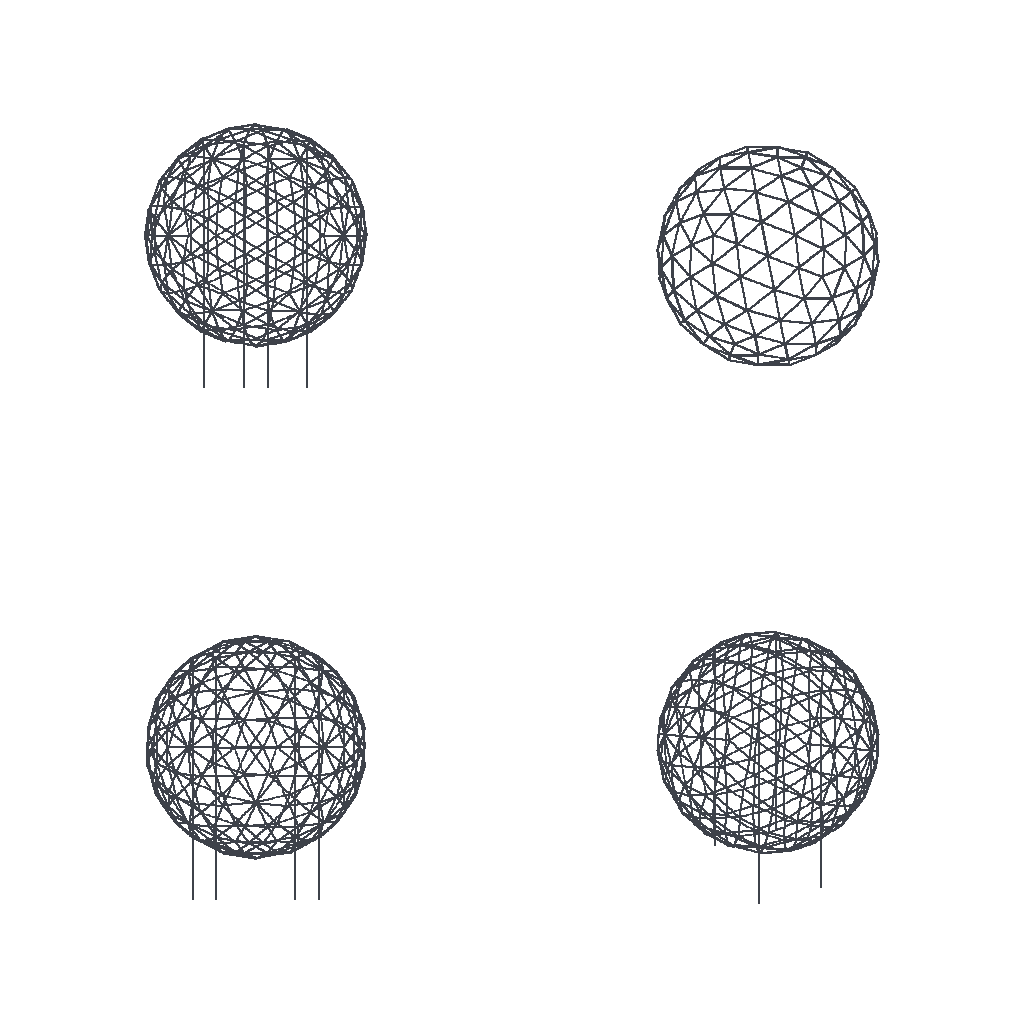Simulation study | abaqus
Set-up summary:
category,name,step,type,value,unit,region
solver,abaqus
solver,version,,,Abaqus/Standard 2020
units,not stated in the deck,,not stated
analysis,deck,,buckling,buckling
load_step,Step-1,Step-1,buckling,nlgeom=False
contact,interactions,,,general=0 pairs=0 ties=0
load_step,requested,,,1
mesh,nodes,,,12925
mesh,elements,,,13240
element_type,B31,,beam,13240
load,load commands in deck,,count,1
bc,support commands in deck,,count,2
material,ALUMINIUM,,in results
material,BPC,,in results
material,BPC_1,,in results
material,Q235,,in results
material,SI_MM111111_Q345,,in results
check,setup vs results,,match,"per instance, exact: element labels, types and connectivity; labels of the nodes the elements use; coordinates of those nodes at SINGLE_PRECISION in 1 of 1 instance(s)"
Abaqus input file, long lists of numbers shortened, first 1045 of 4413 lines:
*Heading
** Job name: Job-1 Model name: Job-4
** Generated by: Abaqus/CAE 2020
*Preprint, echo=NO, model=NO, history=NO, contact=NO
**
** PARTS
**
*Part, name=Part-1
*Node
      1,  -2639.88,     -2027.63,  -1081.56
      2,  -2661.068,  -2001.274,  -1059.834
** (12923 more lines like these left out)
*Element, type=B31
  1, 6026, 6027
  2, 6027, 6028
** (13238 more lines like these left out)
*Nset, nset=_PICKEDSET2_#1, internal
 5761, 5762, 5763, 5764, 5765, 5766, 5767, 5768, 5769, 5770, 5771, 5772, 5773, 5774, 5775, 5776
 5777, 5778, 5779, 5780, 5781, 5782, 5783, 5784, 5785, 5786, 5787, 5788, 5789, 5790, 5791, 5792
** (10 more lines like these left out)
*Elset, elset=_PICKEDSET2_#1, internal, generate
   1,  190,    1
*Nset, nset=_PICKEDSET2_#2, internal
 9114, 9115, 9116, 9117, 9118, 9119, 9120, 9121, 9122, 9123, 9124, 9125, 9126, 9127, 9128, 9129
 9130, 9131, 9132, 9133, 9134, 9135, 9136, 9137, 9138, 9139, 9140, 9141, 9142, 9143, 9144, 9145
** (10 more lines like these left out)
*Elset, elset=_PICKEDSET2_#2, internal, generate
 191,  380,    1
*Nset, nset=_PICKEDSET2_#3, internal
 6823, 6824, 6825, 6826, 6827, 6828, 6829, 6830, 6831, 6832, 6833, 6834, 6835, 6836, 6837, 6838
 6839, 6840, 6841, 6842, 6843, 6844, 6845, 6846, 6847, 6848, 6849, 6850, 6851, 6852, 6853, 6854
** (10 more lines like these left out)
*Elset, elset=_PICKEDSET2_#3, internal, generate
 381,  570,    1
*Nset, nset=_PICKEDSET2_#4, internal
 3484, 3485, 3486, 3487, 3488, 3489, 3490, 3491, 3492, 3493, 3494, 3495, 3496, 3497, 3498, 3499
 3500, 3501, 3502, 3503, 3504, 3505, 3506, 3507, 3508, 3509, 3510, 3511, 3512, 3513, 3514, 3515
** (10 more lines like these left out)
*Elset, elset=_PICKEDSET2_#4, internal, generate
 571,  760,    1
*Nset, nset=SET-1
 6101, 6102, 6103, 6104, 6105, 6106, 6107, 6108, 6109, 6110, 6111, 6112, 6113, 6114, 6115, 6116
 6117, 7798, 7799, 7842, 7843, 7844, 7845, 7846, 7847, 7848, 7849
*Elset, elset=SET-1, generate
 761,  786,    1
*Nset, nset=SET-2
 6166, 6167, 6168, 6169, 6170, 6171, 6172, 6173, 6174, 6175, 6176, 6177, 6178, 6179, 6180, 6181
 6182, 6183, 7842, 7850, 7851, 7852, 7853, 7854, 7855, 7856, 7857
*Elset, elset=SET-2, generate
 787,  812,    1
*Nset, nset=SET-3
 7842, 7858, 7859, 7860, 7861, 7862, 7863, 7864, 7865, 7866, 7867, 7868, 7869, 7870, 7871, 7872
 7873, 7874, 7875, 7876, 7877, 7878, 7879, 7880, 7928, 7929, 7930
*Elset, elset=SET-3, generate
 813,  838,    1
*Nset, nset=SET-4
 7842, 7881, 7882, 7883, 7884, 7885, 7886, 7887, 7888, 7889, 7890, 7891, 7892, 7893, 7894, 7895
 7896, 9659, 9660, 9661, 9662, 9663, 9664, 9665, 9666, 9667, 9668
*Elset, elset=SET-4, generate
 839,  864,    1
*Nset, nset=SET-5
 7661, 7662, 7663, 7800, 7801, 7802, 7803, 7804, 7805, 7806, 7807, 7808, 7809, 7810, 7811, 7812
 7813, 7814, 7815, 7816, 7817, 7818, 7842, 7897, 7898, 7899, 7900
*Elset, elset=SET-5, generate
 865,  890,    1
*Nset, nset=SET-6
 7819, 7820, 7821, 7822, 7823, 7824, 7842, 7901, 7902, 7903, 7904, 7905, 7906, 7907, 7908, 7909
 7910, 9625, 9626, 9627, 9628, 9629, 9630
*Elset, elset=SET-6, generate
 891,  912,    1
*Nset, nset=SET-7
 7663, 7664, 7665, 7666, 7667, 7825, 7826, 7827, 7828, 7829, 7830, 7831, 7832, 7833, 7834, 7835
 9625, 9631, 9632, 9633, 9634, 9635, 9636
*Elset, elset=SET-7, generate
 913,  934,    1
*Nset, nset=SET-8
 9447, 9448, 9449, 9450, 9451, 9452, 9453, 9454, 9455, 9456, 9457, 9458, 9459, 9460, 9461, 9625
 9637, 9638, 9639, 9640, 9641, 9642, 9643
*Elset, elset=SET-8, generate
 935,  956,    1
*Nset, nset=SET-9
  9532,  9533,  9625,  9644,  9645,  9646,  9647,  9648,  9649,  9650,  9651,  9652,  9653,  9654,  9669,  9670
  9671,  9672,  9673,  9674, 11070, 11071, 11072
*Elset, elset=SET-9, generate
 957,  978,    1
*Nset, nset=SET-10
 9625, 9655, 9656, 9657, 9658, 9668, 9675, 9676, 9677, 9678, 9679, 9680, 9681, 9682, 9683, 9684
 9685, 9686, 9687, 9688, 9689, 9690, 9691
*Elset, elset=SET-10, generate
  979,  1000,     1
*Nset, nset=SET-11
  9668,  9692,  9693,  9694,  9695,  9696,  9697,  9698,  9699,  9700,  9701,  9702,  9703,  9704,  9705,  9706
  9707,  9708,  9709,  9710,  9711,  9712, 11070, 11073, 11074, 11300, 11301
*Elset, elset=SET-11, generate
 1001,  1026,     1
*Nset, nset=SET-12
 10081, 10082, 10083, 10084, 10085, 10086, 10087, 10088, 10089, 10371, 10372, 10373, 10374, 10375, 10376, 10377
 10378, 10379, 10380, 11566, 11567, 11568, 11569, 11570, 11571, 11572, 11573, 11574
*Elset, elset=SET-12, generate
 1027,  1053,     1
*Nset, nset=SET-13
 10081, 10090, 10091, 10092, 10093, 10094, 10095, 10096, 10097, 10098, 10099, 10100, 10381, 10382, 10383, 10384
 10385, 10386, 10387, 10388, 10389, 10390, 10391, 10392, 10393, 10394, 10395
*Elset, elset=SET-13, generate
 1054,  1079,     1
*Nset, nset=SET-14
  8460,  8461,  8462,  8463,  8464,  8465,  8466,  8467,  8468,  8469,  8470, 10081, 10101, 10102, 10103, 10104
 10105, 10106, 10107, 10108, 10109, 10110, 10111, 10112, 10113, 10114, 10115, 10116
*Elset, elset=SET-14, generate
 1080,  1106,     1
*Nset, nset=SET-15
  8168,  8169,  8170,  8171,  8172,  8173,  8174,  8175,  8547, 10081, 10117, 10118, 10119, 10120, 10121, 10122
 10126, 10127, 10128, 10129, 10130, 10131, 10132, 10133, 10134, 10135, 10136, 10137
*Elset, elset=SET-15, generate
 1107,  1133,     1
*Nset, nset=SET-16
 11574, 11575, 11576, 11577, 11578, 11599, 11600, 11601, 11602, 11603, 11604, 11605, 11606, 11607, 11608, 11609
 11610, 11611, 11612, 11613, 11614, 11615, 11616, 11617, 11618, 11619, 11620, 11621, 11622
*Elset, elset=SET-16, generate
 1134,  1161,     1
*Nset, nset=SET-17
 10081, 10123, 10124, 10138, 10139, 10140, 10141, 10142, 10143, 10144, 10145, 10146, 10147, 10148, 10149, 11439
 11440, 11441, 11442, 11443, 11444, 11445, 11446, 11447, 11448, 11449, 11450, 11599
*Elset, elset=SET-17, generate
 1162,  1188,     1
*Nset, nset=SET-18
 10081, 10125, 10150, 10151, 10152, 10153, 10154, 10155, 10156, 10157, 10158, 10159, 10160, 10161, 10162, 10163
 10164, 10165, 10166, 10167, 10168, 10169, 10170, 10171, 10172, 10173, 10174
*Elset, elset=SET-18, generate
 1189,  1214,     1
*Nset, nset=SET-19
  8168,  8176,  8177,  8178,  8179,  8180,  8181,  8182,  9958,  9959,  9960,  9961,  9962,  9963,  9964,  9965
  9966,  9967,  9968,  9969,  9970, 10150, 10175, 10176, 10177, 10178, 10179
*Elset, elset=SET-19, generate
 1215,  1240,     1
*Nset, nset=SET-20
 8251, 8252, 8253, 8254, 8255, 8256, 8257, 8258, 8259, 9984, 9985, 9986, 9987, 9988, 9989, 9990
 9991, 9992, 9993, 9994, 9995, 9996, 9997
*Elset, elset=SET-20, generate
 1241,  1262,     1
*Nset, nset=SET-21
  9984,  9998,  9999, 10000, 10001, 10002, 10003, 10004, 10005, 10006, 10007, 10008, 10009, 10010, 10011, 10012
 10013, 10014, 10150, 10180, 10181, 10182, 10183
*Elset, elset=SET-21, generate
 1263,  1284,     1
*Nset, nset=SET-22
 10150, 10184, 10185, 10186, 10187, 10188, 10205, 10206, 10207, 10208, 10209, 10210, 10211, 10212, 10213, 10214
 10215, 10216, 10217, 11469, 11470, 11471, 11472, 11473, 11474, 11475, 11476
*Elset, elset=SET-22, generate
 1285,  1310,     1
*Nset, nset=SET-23
 11451, 11452, 11453, 11454, 11455, 11456, 11457, 11469, 11477, 11478, 11479, 11480, 11481, 11482, 11483, 11484
 11485, 11486, 11487, 11488, 11489, 11490, 11491, 11492, 11493, 11494, 11599
*Elset, elset=SET-23, generate
 1311,  1336,     1
*Nset, nset=SET-24
  9984, 10015, 10016, 10017, 10018, 10019, 10020, 10021, 10022, 10023, 10024, 10046, 10047, 10048, 10049, 10050
 10051, 10052, 10234, 10235, 10236, 10237, 10238
*Elset, elset=SET-24, generate
 1337,  1358,     1
*Nset, nset=SET-25
  8334,  8335,  8336,  8337,  8338,  8339,  8340,  8341,  8342, 10053, 10054, 10055, 10056, 10057, 10058, 10059
 10060, 10061, 10062, 10063, 10064, 10065, 10066, 10067, 10234, 10239, 10240
*Elset, elset=SET-25, generate
 1359,  1384,     1
*Nset, nset=SET-26
 10218, 10219, 10220, 10221, 10222, 10234, 10241, 10242, 10243, 10244, 10245, 10246, 10247, 10248, 10249, 10250
 10251, 10252, 10253, 11469, 11495, 11496, 11497, 11498, 11499, 11500, 11501
*Elset, elset=SET-26, generate
 1385,  1410,     1
*Nset, nset=SET-27
 11469, 11502, 11503, 11504, 11505, 11506, 11507, 11508, 11509, 11510, 11511, 11528, 11529, 11530, 11531, 11532
 11533, 11534, 11535, 11536, 11537, 11538, 11539, 11540, 11541, 11542, 11742
*Elset, elset=SET-27, generate
 1411,  1436,     1
*Nset, nset=SET-28
 11599, 11623, 11624, 11625, 11626, 11627, 11628, 11629, 11661, 11662, 11663, 11664, 11665, 11666, 11667, 11668
 11669, 11670, 11671, 11672, 11673, 11674, 11675, 11676, 11677, 11678, 11679, 11680
*Elset, elset=SET-28, generate
 1437,  1463,     1
*Nset, nset=SET-29
 11661, 11681, 11682, 11683, 11684, 11685, 11686, 11687, 11688, 11689, 11690, 11691, 11692, 11693, 11694, 11695
 11696, 11697, 11896, 11897, 11898, 11899, 11900, 11901, 11902, 11903, 11970, 11971
*Elset, elset=SET-29, generate
 1464,  1490,     1
*Nset, nset=SET-30
 11661, 11698, 11699, 11700, 11701, 11702, 11703, 11704, 11705, 11706, 11707, 11708, 11742, 11743, 11744, 11745
 11746, 11747, 11748, 11749, 11750, 11751, 11752, 11753, 11754, 11755, 11756, 11757
*Elset, elset=SET-30, generate
 1491,  1517,     1
*Nset, nset=SET-31
 11661, 11709, 11710, 11711, 11712, 11713, 11714, 11715, 11716, 11717, 11718, 11719, 11758, 11759, 11760, 11761
 11762, 11763, 12040, 12041, 12042, 12043, 12044, 12045, 12046, 12047, 12048, 12049
*Elset, elset=SET-31, generate
 1518,  1544,     1
*Nset, nset=SET-32
 10234, 10254, 10255, 10256, 10257, 10258, 10259, 10260, 10261, 10262, 10263, 10264, 10265, 10266, 10267, 10268
 10269, 10293, 10294, 10295, 10296, 10297, 10298, 10299, 10300, 10301, 10302
*Elset, elset=SET-32, generate
 1545,  1570,     1
*Nset, nset=SET-33
 10270, 10271, 10272, 10273, 10293, 10303, 10304, 10305, 10306, 10307, 10308, 10309, 10310, 10311, 10312, 11543
 11544, 11545, 11546, 11547, 11548, 11549, 11550, 11551, 11552, 11553, 11554, 11742
*Elset, elset=SET-33, generate
 1571,  1597,     1
*Nset, nset=SET-34
 11742, 11764, 11765, 11766, 11767, 11768, 11769, 11770, 11771, 11772, 11773, 11774, 11775, 11776, 11777, 11778
 11802, 11803, 11804, 11805, 11806, 11807, 11808, 11809, 11810, 11811, 11812, 11813, 11814
*Elset, elset=SET-34, generate
 1598,  1625,     1
*Nset, nset=SET-35
 11742, 11779, 11780, 11781, 11782, 11783, 11784, 11785, 11786, 11787, 11788, 11789, 11790, 11791, 11792, 11793
 11794, 11795, 11796, 11797, 11798, 11799, 11800, 12040, 12050, 12051, 12052, 12053, 12054
*Elset, elset=SET-35, generate
 1626,  1653,     1
*Nset, nset=SET-36
 10234, 10274, 10275, 10276, 10277, 10278, 10279, 10280, 10281, 10282, 10283, 10284, 10285, 10286, 10287, 11555
 11556, 11557, 11558, 11559, 11560, 11561, 11562, 11563, 11564, 11565, 11742
*Elset, elset=SET-36, generate
 1654,  1679,     1
*Nset, nset=SET-37
  8343,  8344,  8345,  8346,  8347,  8419,  8420,  8421, 10068, 10069, 10070, 10071, 10072, 10073, 10074, 10075
 10076, 10077, 10078, 10079, 10080, 10234, 10288, 10289, 10290, 10291, 10292
*Elset, elset=SET-37, generate
 1680,  1705,     1
*Nset, nset=SET-38
 11661, 11720, 11721, 11722, 11723, 11724, 11725, 11726, 11727, 11728, 11972, 11973, 11974, 11975, 11976, 11977
 11978, 11979, 11980, 11981, 11982, 11983, 11984, 11985, 11986, 11987, 11988
*Elset, elset=SET-38, generate
 1706,  1731,     1
*Nset, nset=SET-39
 11469, 11512, 11513, 11514, 11515, 11516, 11517, 11518, 11519, 11520, 11521, 11522, 11523, 11661, 11729, 11730
 11731, 11732, 11733, 11734, 11735, 11736, 11737, 11738, 11739, 11740, 11741
*Elset, elset=SET-39, generate
 1732,  1757,     1
*Nset, nset=SET-40
  9984, 10025, 10026, 10027, 10028, 10029, 10030, 10223, 10224, 10225, 10226, 10227, 10228, 10229, 10230, 10231
 10232, 10233, 11469, 11524, 11525, 11526, 11527
*Elset, elset=SET-40, generate
 1758,  1779,     1
*Nset, nset=SET-41
  8260,  8261,  8262,  8334,  8348,  8349,  8350,  8351,  8352,  9984, 10031, 10032, 10033, 10034, 10035, 10036
 10037, 10038, 10039, 10040, 10041, 10042, 10043
*Elset, elset=SET-41, generate
 1780,  1801,     1
*Nset, nset=SET-42
 11599, 11630, 11631, 11632, 11633, 11634, 11635, 11636, 11637, 11638, 11639, 11640, 11641, 11642, 11643, 11644
 11645, 11646, 11647, 11648, 11649, 11650, 11651, 11903, 11904, 11905, 11906, 11907, 11908
*Elset, elset=SET-42, generate
 1802,  1829,     1
*Nset, nset=SET-43
 10150, 10189, 10190, 10191, 10192, 10193, 10194, 10195, 10196, 10197, 10198, 10199, 10200, 10201, 10202, 11458
 11459, 11460, 11461, 11462, 11463, 11464, 11465, 11466, 11467, 11468, 11599
*Elset, elset=SET-43, generate
 1830,  1855,     1
*Nset, nset=SET-44
  8259,  8263,  8264,  8265,  8266,  8267,  8268,  8269,  8270,  9971,  9972,  9973,  9974,  9975,  9976,  9977
  9978,  9979,  9980,  9981,  9982,  9983, 10044, 10045, 10150, 10203, 10204
*Elset, elset=SET-44, generate
 1856,  1881,     1
*Nset, nset=SET-45
 6183, 6184, 6185, 6186, 6187, 6188, 6189, 6190, 6191, 6192, 6193, 6194, 6195, 6196, 6197, 6198
 6199, 6200, 7911, 7912, 7913, 7914, 7915, 7928, 7931, 7932, 7933, 7934
*Elset, elset=SET-45, generate
 1882,  1908,     1
*Nset, nset=SET-46
  9668,  9713,  9714,  9715,  9716,  9717,  9718,  9719,  9720,  9721,  9722,  9723,  9724,  9725,  9726,  9727
  9728,  9729, 11302, 11303, 11304, 11305, 11328, 11329, 11330, 11331, 11332
*Elset, elset=SET-46, generate
 1909,  1934,     1
*Nset, nset=SET-47
 7916, 7917, 7918, 7919, 7920, 7921, 7922, 7923, 7924, 7925, 7926, 7927, 7928, 7935, 7936, 7937
 7938, 9668, 9730, 9731, 9732, 9733, 9734, 9735, 9736, 9737, 9738
*Elset, elset=SET-47, generate
 1935,  1960,     1
*Nset, nset=SET-48
 9668, 9739, 9740, 9741, 9742, 9743, 9744, 9745, 9746, 9747, 9748, 9749, 9750, 9751, 9752, 9753
 9754, 9755, 9756, 9757, 9758, 9759, 9760, 9761, 9762, 9763, 9764
*Elset, elset=SET-48, generate
 1961,  1986,     1
*Nset, nset=SET-49
  9748,  9765,  9766,  9767,  9768,  9769,  9770,  9771,  9772,  9773,  9774,  9775,  9776,  9777,  9778,  9779
  9780,  9781, 11332, 11333, 11334, 11335, 11336, 11337, 11338, 11339, 11340, 11341
*Elset, elset=SET-49, generate
 1987,  2013,     1
*Nset, nset=SET-50
  9748,  9782,  9783,  9784,  9785,  9786,  9787,  9788,  9789,  9790,  9791,  9792,  9793,  9794,  9795,  9796
  9797,  9798, 11342, 11380, 11381, 11382, 11383, 11384, 11385, 11386, 11387, 11388
*Elset, elset=SET-50, generate
 2014,  2040,     1
*Nset, nset=SET-51
 7928, 7939, 7940, 7941, 7942, 7943, 7944, 7945, 7946, 7947, 7948, 7949, 7950, 7951, 7952, 7953
 7954, 9748, 9799, 9800, 9801, 9802, 9803, 9804, 9805, 9806, 9807, 9808
*Elset, elset=SET-51, generate
 2041,  2067,     1
*Nset, nset=SET-52
 6241, 6242, 6243, 6244, 6245, 6246, 6247, 6248, 6249, 6250, 6251, 6252, 6253, 6254, 6255, 6256
 6257, 6258, 6259, 7928, 7955, 7956, 7957, 7958, 7959, 7960, 7961, 7962, 7963
*Elset, elset=SET-52, generate
 2068,  2095,     1
*Nset, nset=SET-53
 7928, 7964, 7965, 7966, 7967, 7968, 7969, 7970, 7971, 7972, 7973, 7974, 7975, 7976, 7977, 7978
 7979, 7980, 7981, 7982, 7983, 7984, 7985, 7986, 7996, 7997, 7998, 7999, 8000
*Elset, elset=SET-53, generate
 2096,  2123,     1
*Nset, nset=SET-54
 6259, 6260, 6261, 6262, 6263, 6264, 6265, 6266, 6267, 6268, 6269, 6270, 6271, 6272, 6273, 6274
 6275, 6276, 6277, 7987, 7996, 8001, 8002, 8003, 8004, 8005, 8006, 8007, 8008
*Elset, elset=SET-54, generate
 2124,  2151,     1
*Nset, nset=SET-55
 7988, 7989, 7990, 7991, 7992, 7993, 7994, 7995, 7996, 8009, 8010, 8011, 8012, 8013, 8014, 8015
 8016, 9748, 9809, 9810, 9811, 9812, 9813, 9814, 9815, 9816, 9817, 9818
*Elset, elset=SET-55, generate
 2152,  2178,     1
*Nset, nset=SET-56
 9748, 9819, 9820, 9821, 9822, 9823, 9824, 9825, 9826, 9827, 9828, 9829, 9830, 9831, 9832, 9833
 9834, 9835, 9836, 9837, 9838, 9839, 9840, 9841, 9842, 9843, 9844
*Elset, elset=SET-56, generate
 2179,  2204,     1
*Nset, nset=SET-57
  9828,  9845,  9846,  9847,  9848,  9849,  9850,  9851,  9852,  9853,  9854,  9855,  9856,  9857,  9858,  9859
  9860,  9861, 11380, 11389, 11390, 11391, 11392, 11393, 11394, 11395, 11396
*Elset, elset=SET-57, generate
 2205,  2230,     1
*Nset, nset=SET-58
 6315, 6316, 6317, 6318, 6319, 6320, 6321, 6322, 6323, 6324, 6325, 6326, 6327, 6328, 6329, 6330
 6331, 6332, 7996, 8017, 8018, 8019, 8020, 8021, 8022, 8023, 8024, 8025
*Elset, elset=SET-58, generate
 2231,  2257,     1
*Nset, nset=SET-59
 7996, 8026, 8027, 8028, 8029, 8030, 8031, 8032, 8033, 8034, 8035, 8036, 8037, 8038, 8039, 8040
 8041, 8042, 8043, 8044, 8045, 8046, 8047, 8076, 8077, 8078, 8079
*Elset, elset=SET-59, generate
 2258,  2283,     1
*Nset, nset=SET-60
 7996, 8048, 8049, 8050, 8051, 8052, 8053, 8054, 8055, 8056, 8057, 8058, 8059, 8060, 8061, 8062
 8063, 9828, 9862, 9863, 9864, 9865, 9866, 9867, 9868, 9869, 9870
*Elset, elset=SET-60, generate
 2284,  2309,     1
*Nset, nset=SET-61
 8064, 8065, 8066, 8067, 8068, 8069, 8070, 8071, 8072, 8073, 8076, 8080, 8081, 8082, 8083, 8084
 8085, 9828, 9871, 9872, 9873, 9874, 9875, 9876, 9877, 9878, 9879
*Elset, elset=SET-61, generate
 2310,  2335,     1
*Nset, nset=SET-62
 9828, 9880, 9881, 9882, 9883, 9884, 9885, 9886, 9887, 9888, 9889, 9909, 9910, 9911, 9912, 9913
 9914, 9915, 9916, 9917, 9918, 9919, 9920
*Elset, elset=SET-62, generate
 2336,  2357,     1
*Nset, nset=SET-63
  9828,  9890,  9891,  9892,  9893,  9894,  9895,  9896,  9897,  9898,  9899,  9900,  9901,  9902,  9903,  9904
  9905,  9906,  9907,  9908,  9921,  9922, 11224, 11225, 11226, 11437, 11438
*Elset, elset=SET-63, generate
 2358,  2383,     1
*Nset, nset=SET-64
 6462, 6463, 6464, 6465, 6466, 6467, 6468, 6469, 6470, 6471, 8157, 8158, 8159, 8160, 8161, 8162
 8163, 8164, 8165, 8168, 8183, 8184, 8185, 8186, 8187, 8188, 8189, 8190, 8191
*Elset, elset=SET-64, generate
 2384,  2411,     1
*Nset, nset=SET-65
 8166, 8167, 8168, 8192, 8193, 8194, 8195, 8196, 8197, 8470, 8471, 8472, 8473, 8474, 8475, 8476
 8477, 8478, 8479, 8480, 8481, 8482, 8483, 8484, 8485, 8486, 8487, 8488, 8489
*Elset, elset=SET-65, generate
 2412,  2439,     1
*Nset, nset=SET-66
 8334, 8353, 8354, 8355, 8356, 8357, 8358, 8359, 8360, 8361, 8362, 8363, 8364, 8365, 8366, 8367
 8368, 8369, 8370, 8371, 8372, 8373, 8374, 8375, 8376, 8419, 8422
*Elset, elset=SET-66, generate
 2440,  2465,     1
*Nset, nset=SET-67
 6602, 6603, 6604, 6605, 6606, 6607, 6608, 8271, 8272, 8273, 8274, 8275, 8276, 8277, 8278, 8279
 8280, 8281, 8282, 8283, 8334, 8377, 8378, 8379, 8380, 8381, 8382
*Elset, elset=SET-67, generate
 2466,  2491,     1
*Nset, nset=SET-68
 6602, 6609, 6610, 6611, 6612, 6613, 6614, 8259, 8284, 8285, 8286, 8287, 8288, 8289, 8290, 8291
 8292, 8293, 8294, 8295, 8296, 8297, 8298, 8299, 8300, 8301, 8302
*Elset, elset=SET-68, generate
 2492,  2517,     1
*Nset, nset=SET-69
 8168, 8198, 8199, 8200, 8201, 8202, 8203, 8204, 8205, 8206, 8207, 8208, 8209, 8210, 8211, 8212
 8213, 8214, 8215, 8216, 8217, 8218, 8219, 8259, 8303, 8304, 8305
*Elset, elset=SET-69, generate
 2518,  2543,     1
*Nset, nset=SET-70
 8259, 8306, 8307, 8308, 8309, 8310, 8311, 8312, 8313, 8314, 8315, 8316, 8317, 8318, 8319, 8320
 8321, 8322, 8323, 8324, 8325, 8326, 8327, 8334, 8383, 8384, 8385
*Elset, elset=SET-70, generate
 2544,  2569,     1
*Nset, nset=SET-71
 6676, 6677, 6678, 6679, 6680, 6681, 6682, 6683, 8334, 8386, 8387, 8388, 8389, 8390, 8391, 8392
 8393, 8394, 8395, 8396, 8397, 8398, 8399, 8400, 8401, 8402, 8403
*Elset, elset=SET-71, generate
 2570,  2595,     1
*Nset, nset=SET-72
 6527, 6528, 6529, 6530, 6531, 6532, 6533, 6534, 8220, 8221, 8222, 8223, 8224, 8225, 8226, 8227
 8228, 8229, 8230, 8231, 8259, 8328, 8329, 8330, 8331, 8332, 8333
*Elset, elset=SET-72, generate
 2596,  2621,     1
*Nset, nset=SET-73
 6527, 6535, 6536, 6537, 6538, 6539, 6540, 6541, 8168, 8232, 8233, 8234, 8235, 8236, 8237, 8238
 8239, 8240, 8241, 8242, 8243, 8244, 8245, 8246, 8247, 8248, 8249, 8250
*Elset, elset=SET-73, generate
 2622,  2648,     1
*Nset, nset=SET-74
 308, 309, 310, 311, 312, 313, 314, 315, 316, 317, 318, 319, 320, 321, 623, 624
 625, 626, 627, 628, 629, 630, 631, 632, 633, 634, 635
*Elset, elset=SET-74, generate
 2649,  2674,     1
*Nset, nset=SET-75
 308, 322, 323, 324, 325, 326, 327, 328, 329, 330, 331, 332, 333, 334, 335, 336
 337, 338, 339, 340, 341, 342, 343, 344, 345, 393, 394
*Elset, elset=SET-75, generate
 2675,  2700,     1
*Nset, nset=SET-76
 223, 224, 225, 226, 227, 228, 229, 230, 231, 232, 308, 346, 347, 348, 349, 350
 553, 554, 555, 556, 557, 558, 559
*Elset, elset=SET-76, generate
 2701,  2722,     1
*Nset, nset=SET-77
 233, 234, 235, 236, 237, 238, 239, 240, 241, 242, 243, 244, 245, 246, 247, 248
 249, 250, 251, 252, 253, 254, 255, 308, 351, 352, 353
*Elset, elset=SET-77, generate
 2723,  2748,     1
*Nset, nset=SET-78
  32,  33,  34,  35,  36,  37,  38,  39,  40,  41,  42,  43,  44,  45, 256, 257
 258, 259, 260, 261, 308, 354, 355, 356, 357, 358, 359
*Elset, elset=SET-78, generate
 2749,  2774,     1
*Nset, nset=SET-79
  94,  95,  96,  97,  98,  99, 100, 101, 102, 103, 104, 105, 308, 360, 361, 362
 363, 364, 365, 366, 367, 368, 369, 370, 371, 372, 373
*Elset, elset=SET-79, generate
 2775,  2800,     1
*Nset, nset=SET-80
 5696, 5697, 5698, 5699, 5700, 5701, 5702, 7568, 7569, 7570, 7571, 7572, 7573, 7574, 7575, 7576
 7577, 7578, 7579, 7580, 7581, 7582, 7583, 7584, 7585, 7586, 7587, 7588, 7743
*Elset, elset=SET-80, generate
 2801,  2828,     1
*Nset, nset=SET-81
 7461, 7462, 7463, 7464, 7465, 7466, 7589, 7590, 7591, 7592, 7593, 7594, 7595, 7596, 7597, 7598
 7599, 7600, 7601, 7602, 7603, 7604, 7605, 7606, 7607, 7608, 7609, 7610, 7743
*Elset, elset=SET-81, generate
 2829,  2856,     1
*Nset, nset=SET-82
 5702, 5703, 5704, 5705, 5706, 5707, 7461, 7467, 7468, 7469, 7470, 7471, 7472, 7473, 7474, 7475
 7476, 7477, 7478, 7479, 7611, 7612, 7613, 7614, 7615, 7616, 7617, 7618, 7619
*Elset, elset=SET-82, generate
 2857,  2884,     1
*Nset, nset=SET-83
 4379, 4380, 4381, 4382, 4383, 4384, 4385, 4386, 4387, 4388, 4389, 4390, 4391, 4392, 4393, 4394
 4395, 4396, 4397, 4398, 4729, 4730, 4731, 4732, 4733, 4734, 4735, 4736, 4737
*Elset, elset=SET-83, generate
 2885,  2912,     1
*Nset, nset=SET-84
 4729, 4738, 4739, 4740, 4741, 4742, 4743, 4744, 4745, 4746, 4747, 4748, 4749, 4750, 4751, 4752
 4753, 4754, 4755, 6390, 6391, 6392, 6393, 6394, 6395, 6396, 6397, 6398, 6399
*Elset, elset=SET-84, generate
 2913,  2940,     1
*Nset, nset=SET-85
 4398, 4399, 4400, 4401, 4402, 4403, 4404, 4405, 4406, 4407, 4408, 4409, 4410, 4411, 4412, 4413
 4414, 4415, 6017, 6018, 6390, 6400, 6401, 6402, 6403, 6404, 6405, 6406, 6407
*Elset, elset=SET-85, generate
 2941,  2968,     1
*Nset, nset=SET-86
 11332, 11343, 11344, 11345, 11346, 11347, 11348, 11349, 11350, 11351, 11352, 11353, 11354, 11355, 11356, 11357
 11358, 11359, 11360, 11361, 11362, 11363, 11364, 11365, 11380, 11397, 11398, 11399, 11400
*Elset, elset=SET-86, generate
 2969,  2996,     1
*Nset, nset=SET-87
 11149, 11150, 11151, 11152, 11153, 11154, 11155, 11156, 11157, 11158, 11159, 11160, 11161, 11162, 11332, 11366
 11367, 11368, 11369, 11370, 11371, 11372, 11373, 12826, 12827, 12828, 12829, 12830, 12831
*Elset, elset=SET-87, generate
 2997,  3024,     1
*Nset, nset=SET-88
 11163, 11164, 11165, 11166, 11167, 11168, 11169, 11170, 11171, 11172, 11173, 11174, 11175, 11176, 11380, 11401
 11402, 11403, 11404, 11405, 11406, 11407, 11408, 12826, 12832, 12833, 12834, 12835, 12836
*Elset, elset=SET-88, generate
 3025,  3052,     1
*Nset, nset=SET-89
 10802, 10803, 10804, 10805, 10806, 10807, 10954, 10955, 10956, 10957, 10958, 10959, 10960, 10961, 10962, 10963
 10964, 10965, 10966, 10967, 10968, 10969, 10970, 10971, 10972, 10973, 10974, 10975, 11227
*Elset, elset=SET-89, generate
 3053,  3080,     1
*Nset, nset=SET-90
 10976, 10977, 10978, 10979, 10980, 10981, 10982, 10983, 10984, 10985, 10986, 10987, 10988, 10989, 11227, 12755
 12756, 12757, 12758, 12759, 12760, 12761, 12762, 12763, 12764, 12765, 12766, 12767, 12768
*Elset, elset=SET-90, generate
 3081,  3108,     1
*Nset, nset=SET-91
 10807, 10808, 10809, 10810, 10811, 10812, 10813, 10814, 10815, 12439, 12440, 12441, 12442, 12443, 12755, 12769
 12770, 12771, 12772, 12773, 12774, 12775, 12776, 12777, 12778, 12779, 12780, 12781, 12782
*Elset, elset=SET-91, generate
 3109,  3136,     1
*Nset, nset=SET-92
 11801, 11802, 11815, 11816, 11817, 11818, 11819, 11820, 11821, 11822, 11823, 11824, 11825, 11826, 12040, 12055
 12056, 12057, 12058, 12059, 12060, 12061, 12062, 12063, 12064, 12065, 12066, 12067, 12068
*Elset, elset=SET-92, generate
 3137,  3164,     1
*Nset, nset=SET-93
 11574, 11579, 11580, 11581, 11582, 11652, 11653, 11654, 11655, 11656, 11657, 11658, 11659, 11660, 11903, 11909
 11910, 11911, 11912, 11913, 11914, 11915, 11916, 11917, 11918, 11919, 11920, 11921, 11922
*Elset, elset=SET-93, generate
 3165,  3192,     1
*Nset, nset=SET-94
 10744, 10745, 10746, 10747, 10748, 10749, 10750, 10751, 10752, 12169, 12170, 12171, 12172, 12173, 12494, 12495
 12496, 12497, 12498, 12499, 12500, 12501, 12506, 12507, 12508, 12509, 12510, 12511, 12512
*Elset, elset=SET-94, generate
 3193,  3220,     1
*Nset, nset=SET-95
 10885, 10886, 10887, 10888, 10889, 10890, 10891, 10892, 10893, 10894, 10895, 10896, 10897, 10898, 11026, 12502
 12503, 12504, 12505, 12506, 12513, 12514, 12515, 12516, 12517, 12518, 12519, 12520, 12521
*Elset, elset=SET-95, generate
 3221,  3248,     1
*Nset, nset=SET-96
 10752, 10753, 10754, 10755, 10756, 10757, 10899, 10900, 10901, 10902, 10903, 10904, 10905, 10906, 10907, 10908
 10909, 10910, 10911, 10912, 10913, 10914, 10915, 10916, 10917, 10918, 10919, 10920, 11026
*Elset, elset=SET-96, generate
 3249,  3276,     1
*Nset, nset=SET-97
 7412, 7413, 7414, 7415, 7416, 7417, 7510, 7511, 7512, 7513, 7514, 7515, 7516, 7517, 7518, 7519
 7520, 7521, 7522, 7523, 7524, 7525, 7526, 7527, 7528, 7529, 7530, 7531, 7626
*Elset, elset=SET-97, generate
 3277,  3304,     1
*Nset, nset=SET-98
 5631, 5632, 5633, 5634, 5635, 5636, 5637, 7532, 7533, 7534, 7535, 7536, 7537, 7538, 7539, 7540
 7541, 7542, 7543, 7544, 7545, 7546, 7547, 7548, 7549, 7550, 7551, 7552, 7626
*Elset, elset=SET-98, generate
 3305,  3332,     1
*Nset, nset=SET-99
 5129, 5301, 5302, 5303, 5304, 5305, 5306, 5307, 5308, 5309, 5310, 5311, 5312, 5313, 5314, 5315
 5316, 5317, 5318, 5319, 5320, 5321, 5322, 5417, 5418, 5419, 5420, 5421, 5422
*Elset, elset=SET-99, generate
 3333,  3360,     1
*Nset, nset=SET-100
 5129, 5323, 5324, 5325, 5326, 5327, 5328, 5329, 5330, 5331, 5332, 5333, 5334, 5335, 5336, 5337
 5338, 5339, 5340, 5341, 5342, 5343, 7164, 7165, 7166, 7167, 7168, 7169, 7170
*Elset, elset=SET-100, generate
 3361,  3388,     1
*Nset, nset=SET-101
 5344, 5345, 5346, 5347, 5348, 5349, 5350, 5351, 5352, 5422, 5423, 5424, 5425, 5426, 5427, 5428
 5429, 5430, 5431, 5432, 5433, 5434, 5435, 7164, 7171, 7172, 7173, 7174, 7175
*Elset, elset=SET-101, generate
 3389,  3416,     1
*Nset, nset=SET-102
 6471, 6472, 6473, 6474, 6475, 6476, 6477, 6478, 6479, 6946, 6947, 8470, 8490, 8491, 8492, 8493
 8494, 8495, 8496, 8497, 8498, 8499, 8500, 8501, 8502, 8503, 8504, 8505, 8506
*Elset, elset=SET-102, generate
 3417,  3444,     1
*Nset, nset=SET-103
 4900, 4968, 4969, 4970, 4971, 4972, 4973, 4974, 4975, 4976, 6602, 6615, 6616, 6617, 6618, 6619
 6620, 6621, 6622, 6623, 6624, 6625, 6626, 6627, 6628, 6629, 6630, 6631, 6632
*Elset, elset=SET-103, generate
 3445,  3472,     1
*Nset, nset=SET-104
 4901, 4902, 4903, 4904, 4905, 4906, 4907, 4908, 4909, 4910, 6602, 6633, 6634, 6635, 6636, 6637
 6638, 6639, 6640, 6641, 6642, 6643, 6644, 6645, 6646, 6647, 6648, 6649, 6650
*Elset, elset=SET-104, generate
 3473,  3500,     1
*Nset, nset=SET-105
 4901, 4911, 4912, 4913, 4914, 4915, 4916, 4917, 4918, 4919, 4920, 4921, 4922, 4923, 4924, 4925
 4926, 4927, 4928, 4929, 4930, 4931, 4932, 4933, 4976, 4977, 4978, 4979, 4980
*Elset, elset=SET-105, generate
 3501,  3528,     1
*Nset, nset=SET-106
 1516, 1517, 1518, 1519, 1520, 1521, 1522, 1523, 1524, 1525, 1526, 1527, 1528, 1529, 1530, 1531
 1532, 1533, 1534, 1535, 1536, 1537, 1538, 1539, 1568, 1569, 1570, 1571, 1572
*Elset, elset=SET-106, generate
 3529,  3556,     1
*Nset, nset=SET-107
   45,   46,   47,   48,   49,   50, 1516, 1540, 1541, 1542, 1543, 1544, 1545, 1546, 1547, 1750
 1751, 1752, 1753, 1754, 1755, 1756, 1757, 1758, 1759, 1760, 1761, 1762, 1763
*Elset, elset=SET-107, generate
 3557,  3584,     1
*Nset, nset=SET-108
   45,   51,   52,   53,   54,   55, 1572, 1573, 1574, 1575, 1576, 1577, 1578, 1579, 1580, 1764
 1765, 1766, 1767, 1768, 1769, 1770, 1771, 1772, 1773, 1774, 1775, 1776, 1777
*Elset, elset=SET-108, generate
 3585,  3612,     1
*Nset, nset=SET-109
 1825, 1973, 1974, 1975, 1976, 1977, 1978, 1979, 1980, 1981, 1982, 1983, 1984, 1985, 1986, 1987
 1988, 1989, 1990, 1991, 1992, 1993, 1994, 2125, 2126, 2127, 2128, 2129, 2130
*Elset, elset=SET-109, generate
 3613,  3640,     1
*Nset, nset=SET-110
  394,  395,  396,  397,  398,  399,  400,  401,  402,  403,  404,  405,  406,  407, 1825, 1995
 1996, 1997, 1998, 1999, 2000, 2001, 2002, 2003, 2004, 2005, 2006, 2007, 2008
*Elset, elset=SET-110, generate
 3641,  3668,     1
*Nset, nset=SET-111
  394,  408,  409,  410,  411,  412,  413,  414,  415,  416,  417,  418,  419,  420,  421,  703
  704,  705,  706,  707, 2130, 2131, 2132, 2133, 2134, 2135, 2136, 2137, 2138
*Elset, elset=SET-111, generate
 3669,  3696,     1
*Nset, nset=SET-112
 5359, 5360, 5361, 5362, 5363, 5364, 5365, 5366, 5367, 5465, 5466, 5467, 5468, 5469, 5470, 5471
 5472, 5473, 5474, 5475, 5476, 5477, 5478, 7229, 7230, 7231, 7232, 7233, 7234
*Elset, elset=SET-112, generate
 3697,  3724,     1
*Nset, nset=SET-113
 5246, 5368, 5369, 5370, 5371, 5372, 5373, 5374, 5375, 5376, 5377, 5378, 5379, 5380, 5381, 5382
 5383, 5384, 5385, 5386, 5387, 5388, 7229, 7235, 7236, 7237, 7238, 7239, 7240
*Elset, elset=SET-113, generate
 3725,  3752,     1
*Nset, nset=SET-114
 5246, 5389, 5390, 5391, 5392, 5393, 5394, 5395, 5396, 5397, 5398, 5399, 5400, 5401, 5402, 5403
 5404, 5405, 5406, 5407, 5408, 5409, 5410, 5478, 5479, 5480, 5481, 5482, 5483
*Elset, elset=SET-114, generate
 3753,  3780,     1
*Nset, nset=SET-115
 8419, 8423, 8424, 8425, 8426, 8427, 8428, 8429, 8430, 8548, 8549, 8550, 8551, 8552, 8553, 8554
 8555, 8556, 8557, 8558, 8559, 8560, 8561, 8562, 8563, 8564, 8565, 8566, 8567
*Elset, elset=SET-115, generate
 3781,  3808,     1
*Nset, nset=SET-116
 6751, 6752, 6753, 6754, 6755, 6756, 6757, 6758, 6759, 6760, 8419, 8431, 8432, 8433, 8434, 8435
 8436, 8437, 8438, 8439, 8440, 8441, 8442, 8443, 8444, 8445, 8446, 8447, 8448
*Elset, elset=SET-116, generate
 3809,  3836,     1
*Nset, nset=SET-117
 6751, 6761, 6762, 6763, 6764, 6765, 6766, 6767, 6768, 7079, 7080, 8567, 8568, 8569, 8570, 8571
 8572, 8573, 8574, 8575, 8576, 8577, 8578, 8579, 8580, 8581, 8582, 8583, 8584
*Elset, elset=SET-117, generate
 3837,  3864,     1
*Nset, nset=SET-118
  947,  948,  949,  950,  951,  952,  953,  954,  955,  956,  957,  958,  959,  960,  961, 1252
 1312, 1313, 1314, 1315, 1316, 1317, 1318, 1319, 1320, 1321, 1322, 1323, 1324
*Elset, elset=SET-118, generate
 3865,  3892,     1
*Nset, nset=SET-119
  947,  962,  963,  964,  965,  966, 1253, 1254, 1255, 1256, 1257, 1258, 1259, 1260, 1261, 1262
 1263, 1264, 1265, 1266, 1267, 1268, 1269, 1270, 1271, 1272, 1273, 1274, 1275
*Elset, elset=SET-119, generate
 3893,  3920,     1
*Nset, nset=SET-120
 1253, 1276, 1277, 1278, 1279, 1280, 1281, 1282, 1283, 1284, 1285, 1286, 1287, 1288, 1289, 1290
 1324, 1325, 1326, 1327, 1328, 1329, 1330, 1331, 1332, 1333, 1334, 1335, 1336
*Elset, elset=SET-120, generate
 3921,  3948,     1
*Nset, nset=SET-121
 1076, 1077, 1078, 1079, 1080, 1109, 1110, 1111, 1112, 1113, 1114, 1115, 1116, 1117, 1118, 1119
 1120, 1121, 1122, 1123, 1124, 1125, 1126, 1127, 1128, 1129, 1130, 1131, 1132
*Elset, elset=SET-121, generate
 3949,  3976,     1
*Nset, nset=SET-122
  803,  804,  805,  806,  807,  808, 1109, 1133, 1134, 1135, 1136, 1137, 1138, 1139, 1140, 1141
 1142, 1143, 1144, 1145, 1146, 1147, 1148, 1149, 1150, 1151, 1152, 1153, 1154
*Elset, elset=SET-122, generate
 3977,  4004,     1
*Nset, nset=SET-123
  803,  809,  810,  811,  812,  813,  814,  815,  816,  817,  818,  819,  820,  821,  822, 1080
 1081, 1082, 1083, 1084, 1155, 1156, 1157, 1158, 1159, 1160, 1161, 1162, 1163
*Elset, elset=SET-123, generate
 4005,  4032,     1
*Nset, nset=SET-124
 4291, 4292, 4293, 4294, 4295, 4296, 4297, 4298, 4299, 4300, 4301, 4302, 4303, 4304, 4305, 4306
 4307, 4308, 5884, 5885, 6117, 6118, 6119, 6120, 6121, 6122, 6123, 6124, 6125
*Elset, elset=SET-124, generate
 4033,  4060,     1
*Nset, nset=SET-125
 4467, 4468, 4469, 4470, 4471, 4472, 4473, 4474, 4475, 4478, 4479, 4480, 4481, 4482, 4483, 4484
 4485, 4486, 4487, 6117, 6126, 6127, 6128, 6129, 6130, 6131, 6132, 6133, 6134
*Elset, elset=SET-125, generate
 4061,  4088,     1
*Nset, nset=SET-126
 4308, 4309, 4310, 4311, 4312, 4313, 4314, 4315, 4316, 4317, 4318, 4319, 4320, 4321, 4322, 4323
 4324, 4325, 4326, 4327, 4476, 4477, 4478, 4488, 4489, 4490, 4491, 4492, 4493
*Elset, elset=SET-126, generate
 4089,  4116,     1
*Nset, nset=SET-127
  132,  133,  134,  135,  136,  137,  138,  139,  144,  145,  146,  147,  148,  149,  150,  433
  434,  435,  436,  437, 2067, 2068, 2069, 2070, 2071, 2072, 2073, 2074, 2075
*Elset, elset=SET-127, generate
 4117,  4144,     1
*Nset, nset=SET-128
  140,  141,  142,  143,  144,  151,  152,  153,  154,  155,  156,  157,  158,  159, 1627, 1904
 1905, 1906, 1907, 1908, 1909, 1910, 1911, 1912, 1913, 1914, 1915, 1916, 1917
*Elset, elset=SET-128, generate
 4145,  4172,     1
*Nset, nset=SET-129
 1627, 1918, 1919, 1920, 1921, 1922, 1923, 1924, 1925, 1926, 1927, 1928, 1929, 1930, 1931, 1932
 1933, 1934, 1935, 1936, 1937, 1938, 1939, 2075, 2076, 2077, 2078, 2079, 2080
*Elset, elset=SET-129, generate
 4173,  4200,     1
*Nset, nset=SET-130
 4057, 4058, 4059, 4060, 4061, 4062, 4063, 4218, 4219, 4220, 4221, 4222, 4223, 4224, 4225, 4226
 4227, 4228, 4229, 4230, 4231, 4232, 4233
*Elset, elset=SET-130, generate
 4201,  4222,     1
*Nset, nset=SET-131, generate
 4063,  4085,     1
*Elset, elset=SET-131, generate
 4223,  4244,     1
*Nset, nset=SET-132
 7712, 7713, 7714, 7715, 7716, 8086, 8087, 8088, 8089, 8090, 8091, 8092, 8093, 8094, 8095, 8096
 9909, 9923, 9924, 9925, 9926, 9927, 9928
*Elset, elset=SET-132, generate
 4245,  4266,     1
*Nset, nset=SET-133
 9534, 9535, 9536, 9537, 9538, 9539, 9540, 9541, 9542, 9543, 9544, 9545, 9546, 9547, 9548, 9909
 9929, 9930, 9931, 9932, 9933, 9934, 9935
*Elset, elset=SET-133, generate
 4267,  4288,     1
*Nset, nset=SET-134
 8870, 8871, 8872, 8873, 8874, 8875, 8876, 8877, 8878, 8879, 8880, 8881, 8882, 8883, 8884, 8885
 8886, 9036, 9037, 9038, 9039, 9040, 9041
*Elset, elset=SET-134, generate
 4289,  4310,     1
*Nset, nset=SET-135, generate
 8886,  8908,     1
*Elset, elset=SET-135, generate
 4311,  4332,     1
*Nset, nset=SET-136
 2311, 2312, 2313, 2314, 2315, 2512, 2513, 2514, 2515, 2516, 2517, 2518, 2519, 2520, 2521, 2522
 2523, 2524, 2525, 2526, 2527, 4063, 4086
*Elset, elset=SET-136, generate
 4333,  4354,     1
*Nset, nset=SET-137
 2714, 2715, 2716, 2717, 2718, 2872, 2873, 2874, 2875, 2876, 2877, 2878, 2879, 2880, 2881, 2882
 2934, 2935, 2936, 2937, 2938, 2939, 2940
*Elset, elset=SET-137, generate
 4355,  4376,     1
*Nset, nset=SET-138
 2882, 2883, 2884, 2885, 2886, 2887, 2888, 2889, 2890, 2891, 2892, 2893, 2894, 2895, 4561, 4562
 4563, 4644, 4645, 4646, 4647, 4648, 4649
*Elset, elset=SET-138, generate
 4377,  4398,     1
*Nset, nset=SET-139
 8076, 8097, 8098, 8099, 8100, 8101, 8102, 8103, 8104, 8105, 8106, 8107, 8108, 8109, 8110, 8111
 8112, 9909, 9936, 9937, 9938, 9939, 9940
*Elset, elset=SET-139, generate
 4399,  4420,     1
*Nset, nset=SET-140
 2882, 2896, 2897, 2898, 2899, 2900, 2901, 2902, 2903, 2904, 2905, 2906, 2907, 2908, 4564, 4565
 4566, 4567, 4568, 4569, 4570, 4571, 4572
*Elset, elset=SET-140, generate
 4421,  4442,     1
*Nset, nset=SET-141
  9549,  9550,  9909,  9941,  9942,  9943,  9944,  9945,  9946,  9947,  9948,  9949,  9950,  9951,  9952,  9953
  9954,  9955,  9956,  9957, 11224, 11228, 11229
*Elset, elset=SET-141, generate
 4443,  4464,     1
*Nset, nset=SET-142
 12289, 12290, 12291, 12292, 12293, 12294, 12295, 12585, 12586, 12587, 12588, 12589, 12590, 12591, 12592, 12593
 12594, 12595, 12596, 12597, 12598, 12599, 12600
*Elset, elset=SET-142, generate
 4465,  4486,     1
*Nset, nset=SET-143
 12295, 12296, 12297, 12298, 12299, 12300, 12301, 12601, 12602, 12603, 12604, 12605, 12606, 12607, 12608, 12609
 12610, 12670, 12671, 12672, 12673, 12674, 12675
*Elset, elset=SET-143, generate
 4487,  4508,     1
*Nset, nset=SET-144
  8886, 10656, 10657, 10658, 10659, 10660, 10661, 10662, 10663, 10664, 10665, 10666, 10667, 10668, 10669, 10670
 10671, 10672, 10673, 10674, 10675, 10676, 10677
*Elset, elset=SET-144, generate
 4509,  4530,     1
*Nset, nset=SET-145
 12295, 12302, 12303, 12304, 12305, 12306, 12307, 12308, 12309, 12310, 12311, 12359, 12360, 12361, 12362, 12363
 12364, 12365, 12366, 12367, 12368, 12369, 12370
*Elset, elset=SET-145, generate
 4531,  4552,     1
*Nset, nset=SET-146
  8886,  8909, 10501, 10502, 10503, 10504, 10505, 10506, 10507, 10508, 10509, 10510, 10511, 10512, 10513, 10514
 10515, 10516, 10678, 10679, 10680, 10681, 10682
*Elset, elset=SET-146, generate
 4553,  4574,     1
*Nset, nset=SET-147
 11988, 11989, 11990, 11991, 11992, 11993, 12295, 12312, 12313, 12314, 12315, 12316, 12317, 12318, 12319, 12320
 12321, 12322, 12323, 12324, 12325, 12326, 12327
*Elset, elset=SET-147, generate
 4575,  4596,     1
*Nset, nset=SET-148
  8782,  8783, 10366, 10367, 10368, 10369, 10370, 10395, 10396, 10397, 10398, 10399, 10400, 10401, 10402, 10403
 10404, 10405, 10550, 10551, 10552, 10553, 10554
*Elset, elset=SET-148, generate
 4597,  4618,     1
*Nset, nset=SET-149
  8783, 10555, 10556, 10557, 10558, 10559, 10560, 10561, 10562, 10563, 10564, 10565, 10571, 10572, 10573, 10574
 10575, 10576, 10577, 10578, 10579, 10580, 10581
*Elset, elset=SET-149, generate
 4619,  4640,     1
*Nset, nset=SET-150
 12201, 12202, 12203, 12204, 12205, 12295, 12328, 12329, 12330, 12331, 12332, 12333, 12334, 12335, 12336, 12337
 12338, 12339, 12340, 12341, 12342, 12343, 12344
*Elset, elset=SET-150, generate
 4641,  4662,     1
*Nset, nset=SET-151
 8783, 8784, 8785, 8786, 8787, 8788, 8789, 8790, 8791, 8792, 8793, 8794, 8795, 8796, 8797, 8798
 8799, 8958, 8959, 8960, 8961, 8962, 8963
*Elset, elset=SET-151, generate
 4663,  4684,     1
*Nset, nset=SET-152, generate
 3969,  3991,     1
*Elset, elset=SET-152, generate
 4685,  4706,     1
*Nset, nset=SET-153
 3991, 3992, 3993, 3994, 3995, 3996, 3997, 4145, 4146, 4147, 4148, 4149, 4150, 4151, 4152, 4153
 4154, 4155, 4156, 4157, 4158, 4159, 4160
*Elset, elset=SET-153, generate
 4707,  4728,     1
*Nset, nset=SET-154
 8783, 8800, 8801, 8802, 8803, 8804, 8805, 8806, 8807, 8808, 8809, 8810, 8811, 8812, 8813, 8814
 8815, 8816, 8817, 8818, 8819, 8820, 8821
*Elset, elset=SET-154, generate
 4729,  4750,     1
*Nset, nset=SET-155
 3813, 3814, 3815, 3816, 3817, 3818, 3991, 3998, 3999, 4000, 4001, 4002, 4003, 4004, 4005, 4006
 4007, 4008, 4009, 4010, 4011, 4012, 4013
*Elset, elset=SET-155, generate
 4751,  4772,     1
*Nset, nset=SET-156
 2969, 2970, 2971, 2972, 2973, 2974, 2975, 2976, 3306, 3307, 3308, 3309, 3310, 3311, 3312, 3313
 3314, 3315, 3316, 3317, 3318, 3319, 3320
*Elset, elset=SET-156, generate
 4773,  4794,     1
*Nset, nset=SET-157
 2976, 2977, 2978, 2979, 2980, 2981, 2982, 4770, 4771, 4772, 4773, 4774, 4775, 4776, 4777, 4778
 4779, 4780, 5164, 5165, 5166, 5167, 5168
*Elset, elset=SET-157, generate
 4795,  4816,     1
*Nset, nset=SET-158
 8636, 8637, 8638, 8639, 8640, 8641, 8642, 8643, 8644, 8645, 8646, 8647, 8648, 8649, 8650, 8651
 8783, 8822, 8823, 8824, 8825, 8826, 8827
*Elset, elset=SET-158, generate
 4817,  4838,     1
*Nset, nset=SET-159
 2976, 2983, 2984, 2985, 2986, 2987, 4781, 4782, 4783, 4784, 4785, 4786, 4814, 4815, 4816, 4817
 4818, 4819, 4820, 4821, 4822, 4823, 4824
*Elset, elset=SET-159, generate
 4839,  4860,     1
*Nset, nset=SET-160
 3253, 3254, 3255, 3256, 3257, 3258, 5048, 5049, 5050, 5051, 5052, 5053, 5054, 5055, 5056, 5057
 5058, 5059, 5060, 5061, 5062, 5063, 5064
*Elset, elset=SET-160, generate
 4861,  4882,     1
*Nset, nset=SET-161
 3172, 3173, 3174, 3175, 3176, 3177, 3178, 3179, 3180, 3181, 3182, 3258, 3259, 3260, 3261, 3262
 3263, 3264, 3265, 3266, 3267, 3268, 3269
*Elset, elset=SET-161, generate
 4883,  4904,     1
*Nset, nset=SET-162
 2976, 2988, 2989, 2990, 2991, 3003, 3004, 3005, 3006, 3007, 3008, 3009, 3010, 3011, 3012, 3013
 3014, 3015, 3016, 3017, 3018, 3019, 3020
*Elset, elset=SET-162, generate
 4905,  4926,     1
*Nset, nset=SET-163
 1826, 1827, 1828, 3258, 3270, 3271, 3272, 3273, 3274, 3275, 3276, 3277, 3278, 3279, 3280, 3281
 3282, 3283, 3284, 3285, 3286, 3393, 3394
*Elset, elset=SET-163, generate
 4927,  4948,     1
*Nset, nset=SET-164
 1671, 1672, 1673, 2976, 2992, 2993, 2994, 2995, 2996, 2997, 2998, 2999, 3000, 3001, 3002, 3021
 3022, 3023, 3024, 3025, 3026, 3391, 3392
*Elset, elset=SET-164, generate
 4949,  4970,     1
*Nset, nset=SET-165
 255, 262, 263, 264, 265, 266, 267, 268, 269, 270, 271, 272, 273, 274, 275, 276
 559, 560, 561, 562, 563, 564, 565
*Elset, elset=SET-165, generate
 4971,  4992,     1
*Nset, nset=SET-166
 3891, 3892, 3893, 3894, 3895, 3896, 4063, 4087, 4088, 4089, 4090, 4091, 4092, 4093, 4094, 4095
 4096, 4097, 4098, 4099, 4100, 4101, 4102
*Elset, elset=SET-166, generate
 4993,  5014,     1
*Nset, nset=SET-167
 2316, 2317, 2318, 2319, 2320, 2321, 2322, 2323, 2324, 2325, 2326, 2327, 2328, 2329, 2330, 2331
 2332, 2333, 2334, 2335, 2336, 2337, 4063
*Elset, elset=SET-167, generate
 5015,  5036,     1
*Nset, nset=SET-168
 3258, 3287, 3288, 3289, 3290, 3291, 3292, 3293, 3395, 3396, 3397, 3398, 3399, 3400, 3401, 3402
 3403, 3404, 3405, 3406, 3407, 3408, 3409
*Elset, elset=SET-168, generate
 5037,  5058,     1
*Nset, nset=SET-169
 559, 566, 567, 568, 569, 570, 571, 572, 573, 574, 575, 635, 636, 637, 638, 639
 640, 641, 642, 643, 644, 645, 646
*Elset, elset=SET-169, generate
 5059,  5080,     1
*Nset, nset=SET-170
 8709, 8710, 8711, 8712, 8713, 8714, 8715, 8716, 8717, 8718, 8719, 8720, 8721, 8722, 8723, 8724
 8886, 8910, 8911, 8912, 8913, 8914, 8915
*Elset, elset=SET-170, generate
 5081,  5102,     1
*Nset, nset=SET-171
 3258, 3294, 3295, 3296, 3297, 3298, 3299, 5065, 5066, 5067, 5068, 5069, 5070, 5071, 5072, 5073
 5074, 5075, 5215, 5216, 5217, 5218, 5219
*Elset, elset=SET-171, generate
 5103,  5124,     1
*Nset, nset=SET-172
 559, 576, 577, 578, 579, 580, 581, 582, 583, 584, 585, 586, 587, 588, 589, 590
 591, 877, 878, 879, 880, 881, 882
*Elset, elset=SET-172, generate
 5125,  5146,     1
*Nset, nset=SET-173
 1391, 1392, 1393, 1394, 1395, 2685, 2686, 2687, 2688, 2689, 2690, 2691, 2692, 2693, 2694, 2695
 2882, 2909, 2910, 2911, 2912, 2913, 2914
*Elset, elset=SET-173, generate
 5147,  5168,     1
*Nset, nset=SET-174
 2205, 2206, 2207, 2208, 2209, 2377, 2378, 2379, 2380, 2381, 2382, 2383, 2384, 2385, 2386, 2387
 2388, 2389, 2390, 2391, 2392, 3991, 4014
*Elset, elset=SET-174, generate
 5169,  5190,     1
*Nset, nset=SET-175
 2210, 2211, 2212, 2213, 2214, 2215, 2216, 2217, 2218, 2219, 2220, 2226, 2227, 2228, 2229, 2230
 2231, 2232, 2233, 2234, 2235, 2236, 3991
*Elset, elset=SET-175, generate
 5191,  5212,     1
*Nset, nset=SET-176
 2606, 2607, 2608, 2609, 2610, 2882, 2915, 2916, 2917, 2918, 2919, 2920, 2921, 2922, 2923, 2924
 2925, 2926, 2927, 2928, 2929, 2930, 2931
*Elset, elset=SET-176, generate
 5213,  5234,     1
*Nset, nset=SET-177
 465, 466, 467, 468, 469, 559, 592, 593, 594, 595, 596, 597, 598, 599, 600, 601
 602, 603, 604, 605, 606, 607, 608
*Elset, elset=SET-177, generate
 5235,  5256,     1
*Nset, nset=SET-178
 4218, 4234, 4235, 4236, 4237, 4238, 4239, 4240, 5702, 5708, 5709, 5710, 5711, 5712, 5713, 5714
 5715, 5716, 5717, 5718, 5719, 5720, 5721, 5722, 5723, 5724, 5725
*Elset, elset=SET-178, generate
 5257,  5282,     1
*Nset, nset=SET-179
 4064, 4103, 4104, 4105, 5572, 5573, 5574, 5575, 5576, 5577, 5578, 5579, 5580, 5581, 5582, 5583
 5584, 5585, 5586, 5702, 5726, 5727, 5728, 5729, 5730, 5731, 5732
*Elset, elset=SET-179, generate
 5283,  5308,     1
*Nset, nset=SET-180
 7712, 7717, 7718, 7719, 7743, 7744, 7745, 7746, 7747, 7748, 7749, 7750, 7751, 7752, 7753, 7754
 7755, 7756, 7757, 7758, 7759, 7760, 7761, 7762, 7763, 7764, 7765
*Elset, elset=SET-180, generate
 5309,  5334,     1
*Nset, nset=SET-181
 7461, 7480, 7481, 7482, 8887, 8916, 8917, 8918, 8919, 8920, 8921, 8922, 8923, 8924, 9042, 9043
 9044, 9045, 9046, 9047, 9048, 9049, 9050, 9051, 9052, 9053, 9054
*Elset, elset=SET-181, generate
 5335,  5360,     1
*Nset, nset=SET-182
 7743, 7766, 7767, 7768, 7769, 7770, 7771, 7772, 9534, 9551, 9552, 9553, 9602, 9603, 9604, 9605
 9606, 9607, 9608, 9609, 9610, 9611, 9612, 9613, 9614, 9615, 9616
*Elset, elset=SET-182, generate
 5361,  5386,     1
*Nset, nset=SET-183
 7461, 9036, 9055, 9056, 9057, 9058, 9059, 9060, 9061, 9062, 9063, 9064, 9065, 9066, 9067, 9068
 9069, 9070, 9071, 9072, 9073, 9074, 9075, 9076, 9077, 9078, 9079
*Elset, elset=SET-183, generate
 5387,  5412,     1
*Nset, nset=SET-184
 2469, 2512, 2528, 2529, 2530, 2531, 2532, 2533, 2534, 2535, 2536, 2537, 2538, 4398, 4416, 4417
 4418, 4419, 4420, 4421, 4422, 4423, 4424, 4425, 4426, 4427, 4428
*Elset, elset=SET-184, generate
 5413,  5438,     1
*Nset, nset=SET-185
 4218, 4241, 4242, 4243, 4244, 4245, 4246, 4247, 4248, 4249, 4250, 4251, 4252, 4398, 4429, 4430
 4445, 4446, 4447, 4448, 4449, 4450, 4451, 4452, 4453, 4454, 4455
*Elset, elset=SET-185, generate
 5439,  5464,     1
*Nset, nset=SET-186
 2714, 2719, 2720, 2721, 2722, 2723, 2941, 2942, 2943, 2944, 2945, 2946, 2947, 2948, 2949, 2950
 2951, 2952, 2953, 4650, 4651, 4652, 4653, 4654, 4729, 4756, 4757
*Elset, elset=SET-186, generate
 5465,  5490,     1
*Nset, nset=SET-187
 6390, 6408, 6409, 6410, 6411, 6412, 6413, 6414, 6415, 6416, 6417, 6418, 6419, 6420, 6421, 7712
 7720, 7721, 7722, 7723, 7724, 8113, 8114, 8115, 8116, 8117, 8118
*Elset, elset=SET-187, generate
 5491,  5516,     1
*Nset, nset=SET-188
 4644, 4655, 4656, 4657, 4658, 4659, 4660, 4661, 4662, 4663, 4664, 4665, 4666, 4667, 4668, 4669
 4670, 4671, 4672, 4673, 4674, 4675, 4676, 4677, 4678, 4729, 4758
*Elset, elset=SET-188, generate
 5517,  5542,     1
*Nset, nset=SET-189
 6390, 6422, 6423, 6424, 6425, 6426, 6427, 6428, 6429, 6430, 6431, 6432, 6433, 6434, 6435, 6436
 6437, 8076, 8119, 8120, 8121, 8122, 8123, 8124, 8125, 8126, 8127
*Elset, elset=SET-189, generate
 5543,  5568,     1
*Nset, nset=SET-190
 4573, 4574, 4575, 4576, 4577, 4578, 4579, 4580, 4581, 4582, 4583, 4584, 4585, 4644, 4679, 4680
 4681, 4682, 4683, 4684, 6259, 6278, 6279, 6280, 6281, 6282, 6283
*Elset, elset=SET-190, generate
 5569,  5594,     1
*Nset, nset=SET-191
 4564, 4586, 4587, 4588, 4589, 4590, 4591, 4592, 4593, 4594, 4595, 4596, 4597, 4598, 4599, 4600
 4601, 4602, 4603, 4604, 6259, 6284, 6285, 6286, 6287, 6288, 6289
*Elset, elset=SET-191, generate
 5595,  5620,     1
*Nset, nset=SET-192
 11177, 11224, 11230, 11231, 11232, 11380, 11409, 11410, 11411, 11412, 11413, 11414, 11415, 11416, 11417, 11418
 11419, 11420, 11421, 11422, 11423, 11424, 11425, 11426, 11427, 11428, 11429
*Elset, elset=SET-192, generate
 5621,  5646,     1
*Nset, nset=SET-193
 12611, 12612, 12613, 12614, 12615, 12616, 12670, 12676, 12677, 12678, 12679, 12680, 12681, 12826, 12837, 12838
 12839, 12840, 12841, 12842, 12843, 12844, 12845, 12846, 12847, 12848, 12849
*Elset, elset=SET-193, generate
 5647,  5672,     1
*Nset, nset=SET-194
 11070, 11075, 11076, 11077, 11078, 11306, 11307, 11308, 11309, 11310, 11311, 11312, 11313, 11314, 11315, 11316
 11317, 11318, 11319, 11320, 11321, 11322, 11323, 11324, 11332, 11374, 11375
*Elset, elset=SET-194, generate
 5673,  5698,     1
*Nset, nset=SET-195
 12585, 12617, 12618, 12619, 12620, 12621, 12622, 12623, 12624, 12625, 12626, 12627, 12628, 12826, 12850, 12851
 12852, 12853, 12854, 12855, 12856, 12857, 12858, 12859, 12860, 12861, 12862
*Elset, elset=SET-195, generate
 5699,  5724,     1
*Nset, nset=SET-196
  9036, 10807, 10816, 10817, 10842, 10843, 10844, 10845, 10846, 10847, 10848, 10849, 10850, 10851, 10852, 10853
 10854, 10855, 10856, 10857, 10858, 10859, 10860, 10861, 10862, 10863, 10864
*Elset, elset=SET-196, generate
 5725,  5750,     1
*Nset, nset=SET-197
 10656, 10683, 10684, 10685, 10686, 10687, 10688, 10689, 10690, 10691, 10807, 10818, 10819, 10820, 10821, 10822
 10823, 10824, 10825, 10826, 10827, 10828, 10829, 10830, 10831, 10865, 10866
*Elset, elset=SET-197, generate
 5751,  5776,     1
*Nset, nset=SET-198
  9534,  9554,  9555,  9556,  9557,  9558,  9559,  9560,  9561,  9562,  9563,  9564, 11227, 11233, 11234, 11235
 11236, 11237, 11238, 11239, 11240, 11241, 11242, 11243, 11244, 11245, 11246
*Elset, elset=SET-198, generate
 5777,  5802,     1
*Nset, nset=SET-199
 12359, 12371, 12372, 12373, 12374, 12375, 12376, 12377, 12378, 12379, 12380, 12381, 12382, 12383, 12384, 12385
 12386, 12387, 12388, 12682, 12683, 12684, 12685, 12686, 12755, 12783, 12784
*Elset, elset=SET-199, generate
 5803,  5828,     1
*Nset, nset=SET-200
 11224, 11227, 11247, 11248, 11249, 11250, 11251, 11252, 11253, 11254, 11255, 11256, 11257, 11258, 11259, 11260
 11261, 11262, 11263, 11264, 11265, 11266, 11267, 11268, 11269, 11270, 11271
*Elset, elset=SET-200, generate
 5829,  5854,     1
*Nset, nset=SET-201
 12670, 12687, 12688, 12689, 12690, 12691, 12692, 12693, 12694, 12695, 12696, 12697, 12698, 12699, 12700, 12701
 12702, 12703, 12704, 12705, 12706, 12707, 12708, 12709, 12710, 12755, 12785
*Elset, elset=SET-201, generate
 5855,  5880,     1
*Nset, nset=SET-202
 10636, 10637, 10638, 10639, 10640, 10641, 10642, 10643, 10644, 10645, 10646, 10647, 10648, 10656, 10692, 11802
 11827, 11828, 11829, 11830, 11831, 11832, 11833, 12116, 12117, 12118, 12119
Results summary:
result,step,,partial,increments=0 time=0.0/1e-36
result,analysis,,,buckling
result,last_loadstep,,,1
result,analysis steps,,count,1
result,primary field,,,"U, UR"